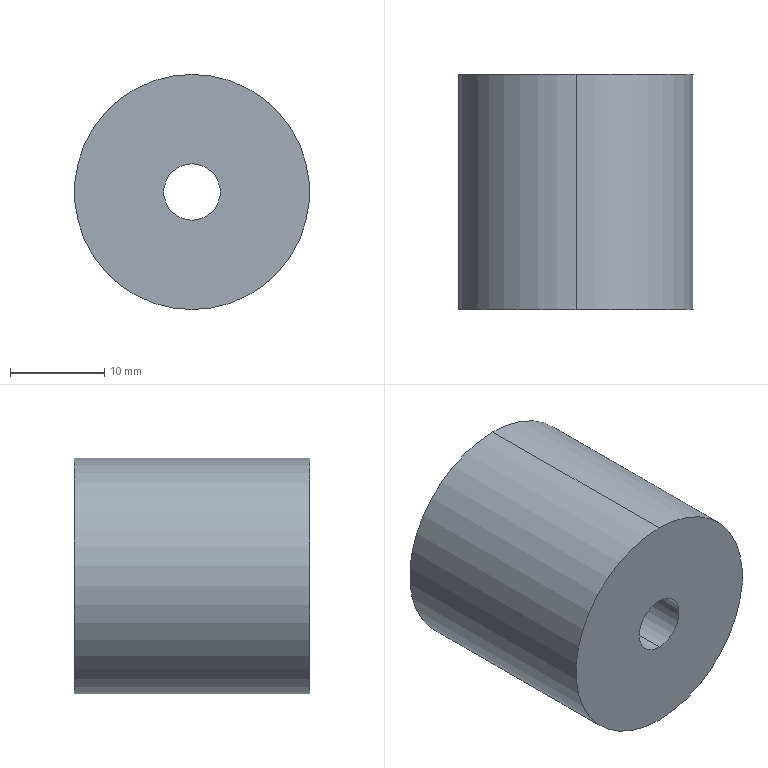Part | SolidWorks | features Extrusion 1 | 1 solid | 6 faces | box 25 x 25 x 25 mm | volume 11565 mm3 | cylinder 4 | plane 2 | commonest cylinder face diameters 6 x2 25 x2
STEP:
#1=CARTESIAN_POINT('',(0.,25.,-3.));
#2=VERTEX_POINT('',#1);
#3=CARTESIAN_POINT('',(0.,25.,3.));
#4=VERTEX_POINT('',#3);
#5=CARTESIAN_POINT('',(0.,25.,0.));
#6=DIRECTION('',(0.,1.,0.));
#7=DIRECTION('',(0.,0.,1.));
#8=AXIS2_PLACEMENT_3D('',#5,#6,#7);
#9=CIRCLE('',#8,3.);
#10=EDGE_CURVE('',#2,#4,#9,.T.);
#11=ORIENTED_EDGE('',*,*,#10,.T.);
#12=CARTESIAN_POINT('',(0.,0.,3.));
#13=VERTEX_POINT('',#12);
#14=CARTESIAN_POINT('',(0.,25.,3.));
#15=DIRECTION('',(0.,-1.,0.));
#16=VECTOR('',#15,1000.);
#17=LINE('',#14,#16);
#18=EDGE_CURVE('',#4,#13,#17,.T.);
#19=ORIENTED_EDGE('',*,*,#18,.T.);
#20=CARTESIAN_POINT('',(0.,0.,-3.));
#21=VERTEX_POINT('',#20);
#22=CARTESIAN_POINT('',(0.,0.,0.));
#23=DIRECTION('',(0.,1.,0.));
#24=DIRECTION('',(0.,0.,1.));
#25=AXIS2_PLACEMENT_3D('',#22,#23,#24);
#26=CIRCLE('',#25,3.);
#27=EDGE_CURVE('',#21,#13,#26,.T.);
#28=ORIENTED_EDGE('',*,*,#27,.F.);
#29=CARTESIAN_POINT('',(0.,25.,-3.));
#30=DIRECTION('',(0.,-1.,0.));
#31=VECTOR('',#30,1000.);
#32=LINE('',#29,#31);
#33=EDGE_CURVE('',#2,#21,#32,.T.);
#34=ORIENTED_EDGE('',*,*,#33,.F.);
#35=EDGE_LOOP('',(#11,#19,#28,#34));
#36=FACE_OUTER_BOUND('',#35,.T.);
#37=CARTESIAN_POINT('',(0.,25.,0.));
#38=DIRECTION('',(0.,-1.,0.));
#39=DIRECTION('',(0.,0.,-1.));
#40=AXIS2_PLACEMENT_3D('',#37,#38,#39);
#41=CYLINDRICAL_SURFACE('',#40,3.);
#42=ADVANCED_FACE('',(#36),#41,.F.);
#43=CARTESIAN_POINT('',(0.,25.,12.5));
#44=VERTEX_POINT('',#43);
#45=CARTESIAN_POINT('',(0.,25.,-12.5));
#46=VERTEX_POINT('',#45);
#47=CARTESIAN_POINT('',(0.,25.,0.));
#48=DIRECTION('',(0.,1.,0.));
#49=DIRECTION('',(0.,0.,1.));
#50=AXIS2_PLACEMENT_3D('',#47,#48,#49);
#51=CIRCLE('',#50,12.5);
#52=EDGE_CURVE('',#44,#46,#51,.T.);
#53=ORIENTED_EDGE('',*,*,#52,.F.);
#54=CARTESIAN_POINT('',(0.,0.,12.5));
#55=VERTEX_POINT('',#54);
#56=CARTESIAN_POINT('',(0.,25.,12.5));
#57=DIRECTION('',(0.,-1.,0.));
#58=VECTOR('',#57,1000.);
#59=LINE('',#56,#58);
#60=EDGE_CURVE('',#44,#55,#59,.T.);
#61=ORIENTED_EDGE('',*,*,#60,.T.);
#62=CARTESIAN_POINT('',(0.,0.,-12.5));
#63=VERTEX_POINT('',#62);
#64=CARTESIAN_POINT('',(0.,0.,0.));
#65=DIRECTION('',(0.,1.,0.));
#66=DIRECTION('',(0.,0.,1.));
#67=AXIS2_PLACEMENT_3D('',#64,#65,#66);
#68=CIRCLE('',#67,12.5);
#69=EDGE_CURVE('',#55,#63,#68,.T.);
#70=ORIENTED_EDGE('',*,*,#69,.T.);
#71=CARTESIAN_POINT('',(0.,25.,-12.5));
#72=DIRECTION('',(0.,-1.,0.));
#73=VECTOR('',#72,1000.);
#74=LINE('',#71,#73);
#75=EDGE_CURVE('',#46,#63,#74,.T.);
#76=ORIENTED_EDGE('',*,*,#75,.F.);
#77=EDGE_LOOP('',(#53,#61,#70,#76));
#78=FACE_OUTER_BOUND('',#77,.T.);
#79=CARTESIAN_POINT('',(0.,25.,0.));
#80=DIRECTION('',(0.,-1.,0.));
#81=DIRECTION('',(0.,0.,-1.));
#82=AXIS2_PLACEMENT_3D('',#79,#80,#81);
#83=CYLINDRICAL_SURFACE('',#82,12.5);
#84=ADVANCED_FACE('',(#78),#83,.T.);
#85=CARTESIAN_POINT('',(0.,25.,0.));
#86=DIRECTION('',(0.,1.,0.));
#87=DIRECTION('',(0.,0.,1.));
#88=AXIS2_PLACEMENT_3D('',#85,#86,#87);
#89=CIRCLE('',#88,12.5);
#90=EDGE_CURVE('',#46,#44,#89,.T.);
#91=ORIENTED_EDGE('',*,*,#90,.T.);
#92=ORIENTED_EDGE('',*,*,#52,.T.);
#93=EDGE_LOOP('',(#91,#92));
#94=FACE_OUTER_BOUND('',#93,.T.);
#95=ORIENTED_EDGE('',*,*,#10,.F.);
#96=CARTESIAN_POINT('',(0.,25.,0.));
#97=DIRECTION('',(0.,1.,0.));
#98=DIRECTION('',(0.,0.,1.));
#99=AXIS2_PLACEMENT_3D('',#96,#97,#98);
#100=CIRCLE('',#99,3.);
#101=EDGE_CURVE('',#4,#2,#100,.T.);
#102=ORIENTED_EDGE('',*,*,#101,.F.);
#103=EDGE_LOOP('',(#95,#102));
#104=FACE_BOUND('',#103,.T.);
#105=CARTESIAN_POINT('',(0.,25.,0.));
#106=DIRECTION('',(0.,1.,0.));
#107=DIRECTION('',(0.,0.,1.));
#108=AXIS2_PLACEMENT_3D('',#105,#106,#107);
#109=PLANE('',#108);
#110=ADVANCED_FACE('',(#94,#104),#109,.T.);
#111=CARTESIAN_POINT('',(0.,0.,0.));
#112=DIRECTION('',(0.,1.,0.));
#113=DIRECTION('',(0.,0.,1.));
#114=AXIS2_PLACEMENT_3D('',#111,#112,#113);
#115=CIRCLE('',#114,12.5);
#116=EDGE_CURVE('',#63,#55,#115,.T.);
#117=ORIENTED_EDGE('',*,*,#116,.F.);
#118=ORIENTED_EDGE('',*,*,#69,.F.);
#119=EDGE_LOOP('',(#117,#118));
#120=FACE_OUTER_BOUND('',#119,.T.);
#121=ORIENTED_EDGE('',*,*,#27,.T.);
#122=CARTESIAN_POINT('',(0.,0.,0.));
#123=DIRECTION('',(0.,1.,0.));
#124=DIRECTION('',(0.,0.,1.));
#125=AXIS2_PLACEMENT_3D('',#122,#123,#124);
#126=CIRCLE('',#125,3.);
#127=EDGE_CURVE('',#13,#21,#126,.T.);
#128=ORIENTED_EDGE('',*,*,#127,.T.);
#129=EDGE_LOOP('',(#121,#128));
#130=FACE_BOUND('',#129,.T.);
#131=CARTESIAN_POINT('',(0.,0.,0.));
#132=DIRECTION('',(0.,1.,0.));
#133=DIRECTION('',(0.,0.,1.));
#134=AXIS2_PLACEMENT_3D('',#131,#132,#133);
#135=PLANE('',#134);
#136=ADVANCED_FACE('',(#120,#130),#135,.F.);
#137=ORIENTED_EDGE('',*,*,#60,.F.);
#138=ORIENTED_EDGE('',*,*,#90,.F.);
#139=ORIENTED_EDGE('',*,*,#75,.T.);
#140=ORIENTED_EDGE('',*,*,#116,.T.);
#141=EDGE_LOOP('',(#137,#138,#139,#140));
#142=FACE_OUTER_BOUND('',#141,.T.);
#143=CARTESIAN_POINT('',(0.,25.,0.));
#144=DIRECTION('',(0.,-1.,0.));
#145=DIRECTION('',(0.,0.,-1.));
#146=AXIS2_PLACEMENT_3D('',#143,#144,#145);
#147=CYLINDRICAL_SURFACE('',#146,12.5);
#148=ADVANCED_FACE('',(#142),#147,.T.);
#149=ORIENTED_EDGE('',*,*,#18,.F.);
#150=ORIENTED_EDGE('',*,*,#101,.T.);
#151=ORIENTED_EDGE('',*,*,#33,.T.);
#152=ORIENTED_EDGE('',*,*,#127,.F.);
#153=EDGE_LOOP('',(#149,#150,#151,#152));
#154=FACE_OUTER_BOUND('',#153,.T.);
#155=CARTESIAN_POINT('',(0.,25.,0.));
#156=DIRECTION('',(0.,-1.,0.));
#157=DIRECTION('',(0.,0.,-1.));
#158=AXIS2_PLACEMENT_3D('',#155,#156,#157);
#159=CYLINDRICAL_SURFACE('',#158,3.);
#160=ADVANCED_FACE('',(#154),#159,.F.);
#161=CLOSED_SHELL('',(#42,#84,#110,#136,#148,#160));
#162=MANIFOLD_SOLID_BREP('',#161);
#163=CARTESIAN_POINT('',(0.,0.,0.));
#164=DIRECTION('',(0.,0.,1.));
#165=DIRECTION('',(1.,0.,0.));
#166=AXIS2_PLACEMENT_3D('',#163,#164,#165);
#167=(LENGTH_UNIT()NAMED_UNIT(*)SI_UNIT(.MILLI.,.METRE.));
#168=UNCERTAINTY_MEASURE_WITH_UNIT(LENGTH_MEASURE(0.00001),#167,'','');
#169=(NAMED_UNIT(*)PLANE_ANGLE_UNIT()SI_UNIT($,.RADIAN.));
#170=(NAMED_UNIT(*)SI_UNIT($,.STERADIAN.)SOLID_ANGLE_UNIT());
#171=(GEOMETRIC_REPRESENTATION_CONTEXT(3)GLOBAL_UNCERTAINTY_ASSIGNED_CONTEXT((#168))GLOBAL_UNIT_ASSIGNED_CONTEXT((#167,#169,#170))REPRESENTATION_CONTEXT('',''));
#172=ADVANCED_BREP_SHAPE_REPRESENTATION('',(#162,#166),#171);